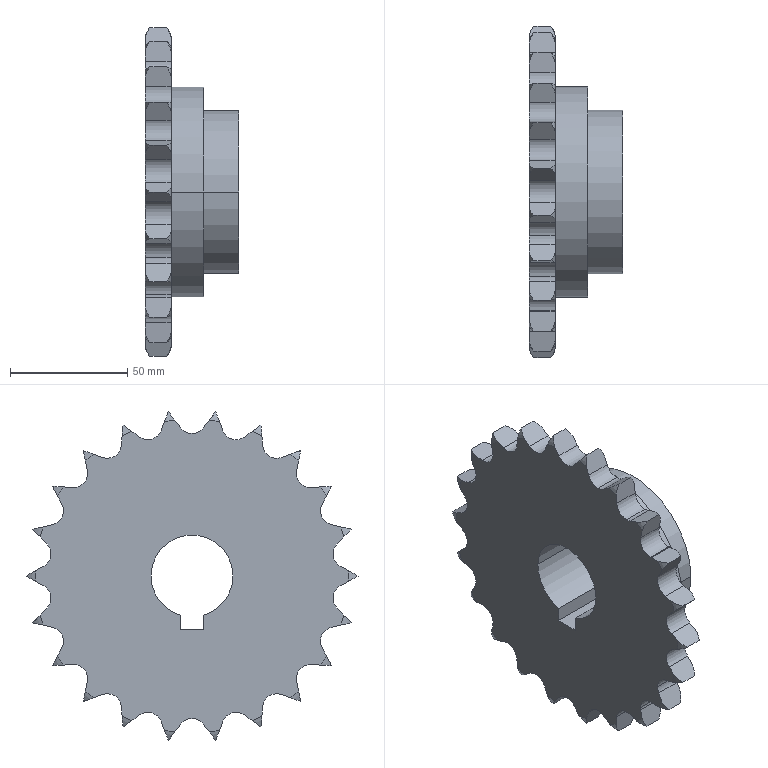Part | STEP file | IN-01-09-02 | 1 solid | 129 faces | box 40 x 141.8 x 140.357 mm | volume 249105 mm3 | plane 51 | spline 44 | cylinder 34 | commonest cylinder face diameters 12.07 x27 35 x3 70 x2 90 x2